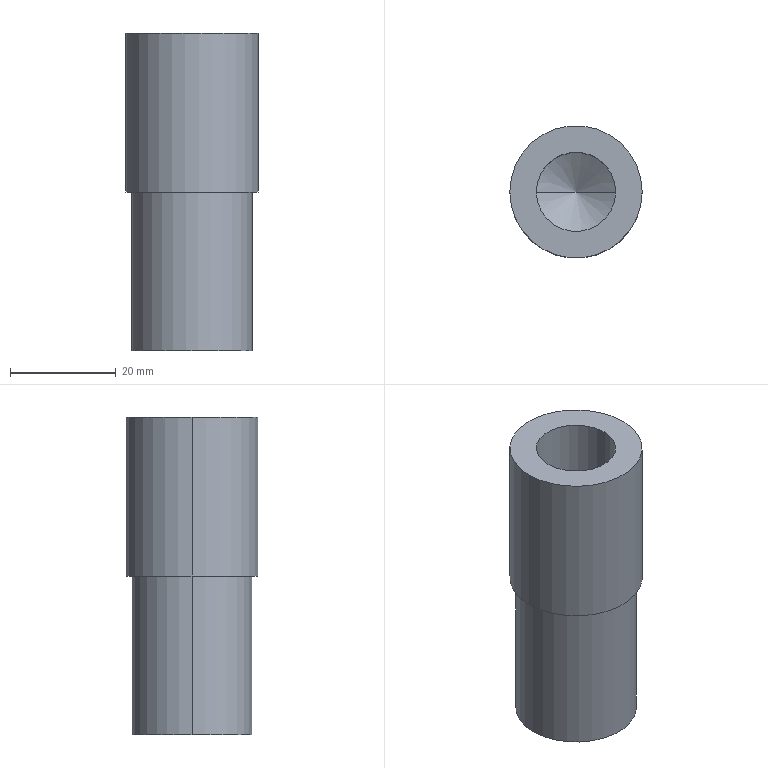Part | SolidWorks | features Extrusion 1, ICE 1, RevCut 1 | 1 solid | 11 faces | box 25 x 25 x 60 mm | volume 21851 mm3 | cylinder 6 | plane 3 | cone 2 | commonest cylinder face diameters 15 x2 22.8 x2 25 x2